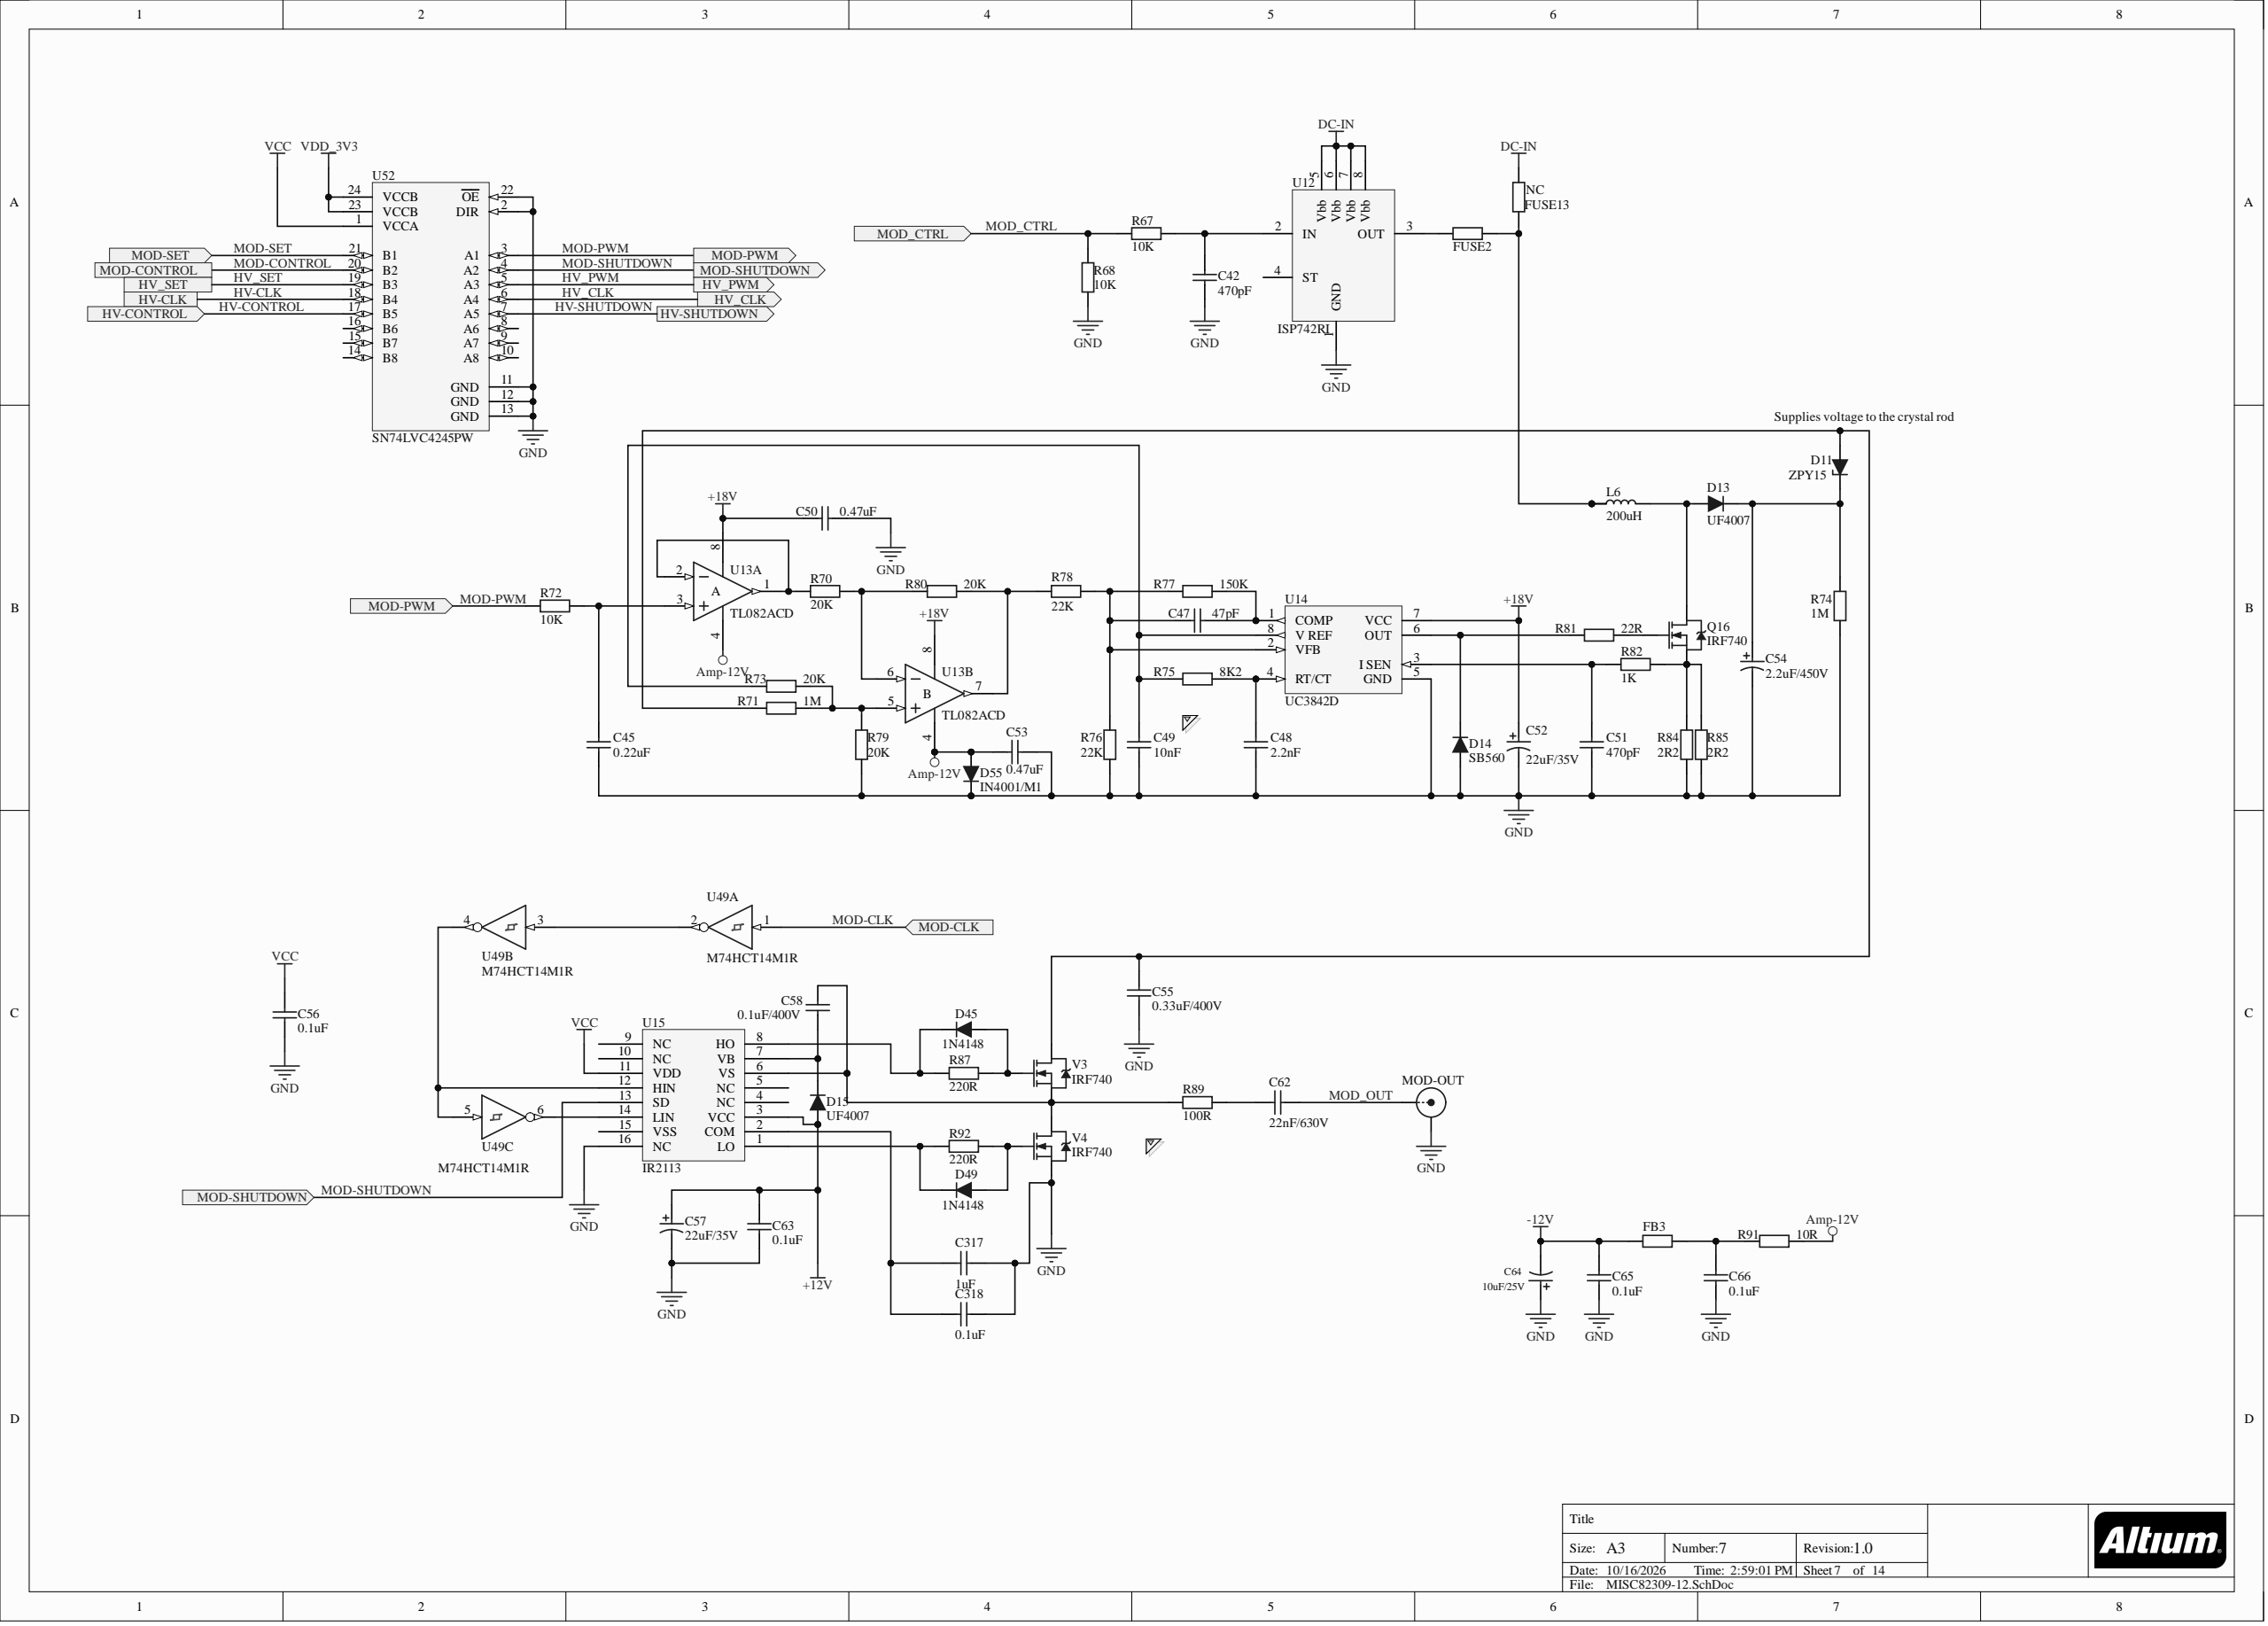Circuit board | Altium Designer | 747 parts | 576 nets | one sheet of the schematic
Parts on this sheet (reference | value | footprint):
C42 | 470pF | C0603
C45 | 0.22uF | C1206
C47 | 47pF | C1206
C48 | 2.2nF | C1206
C49 | 10nF | C1206
C50 | 0.47uF | C1206
C51 | 470pF | C1206
C52 | 22uF/35V | E6.3X5.4
C53 | 0.47uF | C1206
C54 | 2.2uF/450V | CAP-EL-10X13_5-5
C55 | 0.33uF/400V | CBB-400V-10mm
C56 | 0.1uF | CAP_0805
C57 | 22uF/35V | CAP_AVX-A
C58 | 0.1uF/400V | CBB-400V-10mm
C62 | 22nF/630V | CBB-400V-10mm
C63 | 0.1uF | C1206
C64 | 10uF/25V | E5X5.4
C65 | 0.1uF | C0805
C66 | 0.1uF | C0805
C317 | 1uF | CAP_0805
C318 | 0.1uF | CAP_0805
D11 | ZPY15 | DO-41 - 10.46mm
D13 | UF4007 | DO-41 - 10.46mm
D14 | SB560 | DO-201AD
D15 | UF4007 | DO-41 - 10.46mm
D45 | 1N4148 | DO-213AA
D49 | 1N4148 | DO-213AA
D55 | IN4001/M1 | DO-214AC
FB3 | 60 | SMD0805-L
FUSE2 | ASMD050-1812(30V,0.5A) | SMD1812-Fuse
FUSE13 | ASMD050-1812(30V,0.5A) | SMD1812-Fuse
L6 | 200uH | L200/1.4A
MOD-OUT | SMB | SMB_V-RJ45
Q16 | IRF740 | TO220V1
R67 | 10K | R0603
R68 | 10K | R0603
R70 | 20K | R1206
R71 | 1M | R1206
R72 | 10K | R1206
R73 | 20K | R1206
R74 | 1M | R1206
R75 | 8K2 | R1206
R76 | 22K | R1206
R77 | 150K | R1206
R78 | 22K | R1206
R79 | 20K | R1206
R80 | 20K | R1206
R81 | 22R | R1206
R82 | 1K | R1206
R84 | 2R2 | R1206
R85 | 2R2 | R1206
R87 | 220R | R1206
R89 | 100R | RES_2512
R91 | 10R | RES_0805
R92 | 220R | R1206
U12 | ISP742RI | P-DSO-8
U14 | UC3842D | SOIC-8
U15 | IR2113 | SOIC-16
U52 | SN74LVC4245PW | TSSOP-24
V3 | IRF740 | TO220V1
V4 | IRF740 | TO220V1
Nets of these parts (net: part-pin ...):
VDD_3V3: U52-23 U52-24
VCC: C56-1 U15-11 U52-1
NetU15_14: U15-14
NetU15_12: U15-12
NetR78_1: R78-1 R80-2
NetR71_2: R71-2 R73-2 R79-2
NetR70_2: R70-2 R80-1
NetR70_1: R70-1
NetQ16_3: Q16-3 R82-2 R84-2 R85-2
NetQ16_1: Q16-1 R81-2
NetFUSE2_2: FUSE2-2 FUSE13-2 L6-1 L6-3
NetFUSE2_1: FUSE2-1 U12-3
NetD49_2: D49-2 R92-2 U15-1
NetD49_1: D49-1 R92-1 V4-1
NetD45_2: D45-2 R87-2 U15-8
NetD45_1: D45-1 R87-1 V3-1
NetD14_2: D14-2 R81-1 U14-6
NetD13_1: D13-1 L6-2 Q16-2
NetC317_1: C317-1 C318-1 U15-2
NetC66_2: C66-2 FB3-2 R91-1
NetC62_1: C62-1 R89-2
NetC58_2: C58-2 D15-2 U15-7
NetC58_1: C58-1 R89-1 U15-6 V3-3 V4-2
NetC55_2: C55-2 D11-1 R71-1 V3-2
NetC54_1: C54-1 D11-2 D13-2 R74-2
NetC51_1: C51-1 R82-1 U14-3
NetC49_1: C49-1 R73-1 R75-1 U14-8
NetC48_1: C48-1 R75-2 U14-4
NetC47_2: C47-2 R76-2 R77-1 R78-2 U14-2
NetC47_1: C47-1 R77-2 U14-1
NetC45_1: C45-1 R72-1
NetC42_2: C42-2 R67-1 U12-2
MOD_OUT: C62-2 MOD-OUT-1
MOD_CTRL: R67-2 R68-2
MOD-SHUTDOWN: U15-13 U52-4
MOD-SET: U52-21
MOD-PWM: R72-2 U52-3
MOD-CONTROL: U52-20
HV_SET: U52-19
HV_PWM: U52-5
HV_CLK: U52-6
HV-SHUTDOWN: U52-7
HV-CONTROL: U52-17
HV-CLK: U52-18
GND: C42-1 C45-2 C48-2 C49-2 C50-2 C51-2 C52-2 C53-2 C54-2 C55-1 C56-2 C57-2 C63-1 C64-1 C65-1 C66-1 C317-2 C318-2 D14-1 D55-2 MOD-OUT-2 R68-1 R74-1 R76-1 R79-1 R84-1 R85-1 U12-1 U14-5 U15-16 U52-2 U52-11 U52-12 U52-13 U52-22 V4-3
DC-IN: FUSE13-1 U12-5 U12-6 U12-7 U12-8
Amp-12V: C53-1 D55-1 R91-2
-12V: C64-2 C65-2 FB3-1
+18V: C50-1 C52-1 U14-7
+12V: C57-1 C63-2 D15-1 U15-3